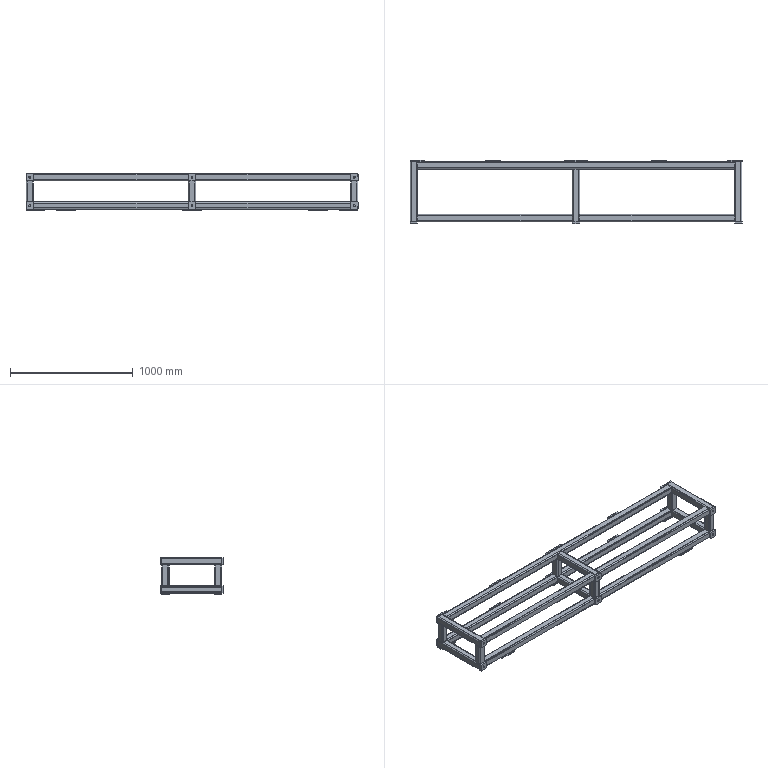Part | SolidWorks | features HoleWzd 9, WeldCornerFeat 6, ICE 4, WeldMemberFeat 3, 3DProfileFeature 1, WeldmentFeature 1 | 39 solids | 654 faces | box 2700 x 516 x 300 mm | volume 16210960 mm3 | plane 390 | cylinder 260 | cone 4 | commonest cylinder face diameters 10 x72 20 x72 6.8 x48 10.2 x40 4.2 x16 14 x12